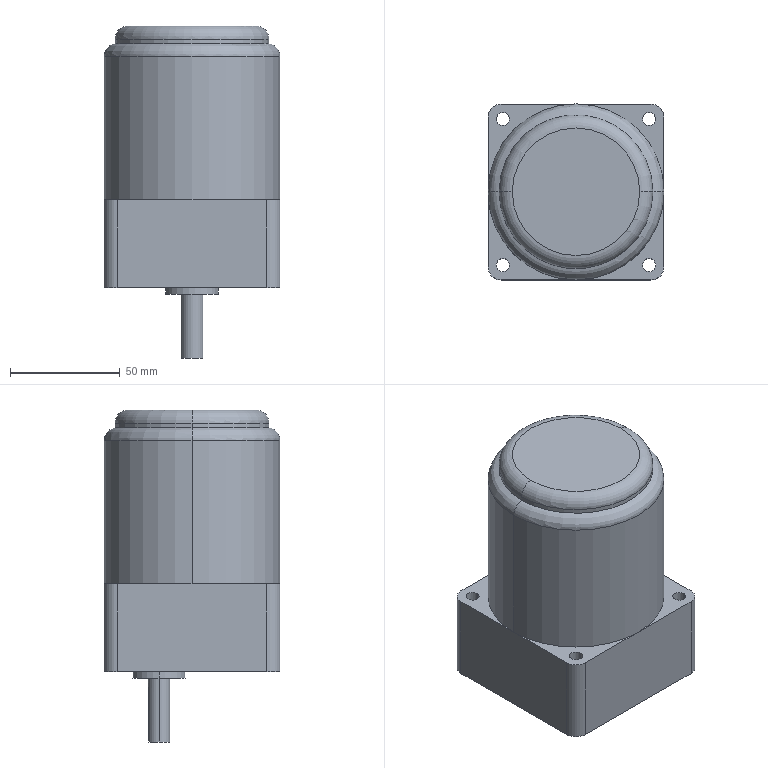Part | STEP file | 1 solid | 40 faces | box 80 x 80 x 151 mm | volume 637905 mm3 | cylinder 20 | plane 16 | torus 4 | commonest cylinder face diameters 6 x8 12 x4 10 x2 24 x2 70 x2 80 x2
STEP:
#1=CARTESIAN_POINT('',(34.,-40.,40.));
#2=VERTEX_POINT('',#1);
#3=CARTESIAN_POINT('',(0.,-40.,40.));
#4=VERTEX_POINT('',#3);
#5=CARTESIAN_POINT('',(34.,-40.,40.));
#6=DIRECTION('',(-1.,0.,0.));
#7=VECTOR('',#6,1000.);
#8=LINE('',#5,#7);
#9=EDGE_CURVE('',#2,#4,#8,.T.);
#10=ORIENTED_EDGE('',*,*,#9,.F.);
#11=CARTESIAN_POINT('',(40.,-34.,40.));
#12=VERTEX_POINT('',#11);
#13=CARTESIAN_POINT('',(34.,-34.,40.));
#14=DIRECTION('',(0.,0.,1.));
#15=DIRECTION('',(0.,-1.,0.));
#16=AXIS2_PLACEMENT_3D('',#13,#14,#15);
#17=CIRCLE('',#16,6.);
#18=EDGE_CURVE('',#2,#12,#17,.T.);
#19=ORIENTED_EDGE('',*,*,#18,.T.);
#20=CARTESIAN_POINT('',(40.,0.,40.));
#21=VERTEX_POINT('',#20);
#22=CARTESIAN_POINT('',(40.,0.,40.));
#23=DIRECTION('',(0.,-1.,0.));
#24=VECTOR('',#23,1000.);
#25=LINE('',#22,#24);
#26=EDGE_CURVE('',#21,#12,#25,.T.);
#27=ORIENTED_EDGE('',*,*,#26,.F.);
#28=CARTESIAN_POINT('',(0.,0.,40.));
#29=DIRECTION('',(0.,0.,-1.));
#30=DIRECTION('',(1.,0.,0.));
#31=AXIS2_PLACEMENT_3D('',#28,#29,#30);
#32=CIRCLE('',#31,40.);
#33=EDGE_CURVE('',#21,#4,#32,.T.);
#34=ORIENTED_EDGE('',*,*,#33,.T.);
#35=EDGE_LOOP('',(#10,#19,#27,#34));
#36=FACE_OUTER_BOUND('',#35,.T.);
#37=CARTESIAN_POINT('',(36.234,-33.234,40.));
#38=VERTEX_POINT('',#37);
#39=CARTESIAN_POINT('',(30.234,-33.234,40.));
#40=VERTEX_POINT('',#39);
#41=CARTESIAN_POINT('',(33.234,-33.234,40.));
#42=DIRECTION('',(0.,0.,-1.));
#43=DIRECTION('',(1.,0.,0.));
#44=AXIS2_PLACEMENT_3D('',#41,#42,#43);
#45=CIRCLE('',#44,3.);
#46=EDGE_CURVE('',#38,#40,#45,.T.);
#47=ORIENTED_EDGE('',*,*,#46,.T.);
#48=CARTESIAN_POINT('',(33.234,-33.234,40.));
#49=DIRECTION('',(0.,0.,-1.));
#50=DIRECTION('',(-1.,0.,0.));
#51=AXIS2_PLACEMENT_3D('',#48,#49,#50);
#52=CIRCLE('',#51,3.);
#53=EDGE_CURVE('',#40,#38,#52,.T.);
#54=ORIENTED_EDGE('',*,*,#53,.T.);
#55=EDGE_LOOP('',(#47,#54));
#56=FACE_BOUND('',#55,.T.);
#57=CARTESIAN_POINT('',(-1.06,-41.06,40.));
#58=DIRECTION('',(0.,0.,1.));
#59=DIRECTION('',(1.,0.,0.));
#60=AXIS2_PLACEMENT_3D('',#57,#58,#59);
#61=PLANE('',#60);
#62=ADVANCED_FACE('',(#36,#56),#61,.T.);
#63=CARTESIAN_POINT('',(34.,-40.,0.));
#64=VERTEX_POINT('',#63);
#65=CARTESIAN_POINT('',(-34.,-40.,0.));
#66=VERTEX_POINT('',#65);
#67=CARTESIAN_POINT('',(34.,-40.,0.));
#68=DIRECTION('',(-1.,0.,0.));
#69=VECTOR('',#68,1000.);
#70=LINE('',#67,#69);
#71=EDGE_CURVE('',#64,#66,#70,.T.);
#72=ORIENTED_EDGE('',*,*,#71,.F.);
#73=CARTESIAN_POINT('',(34.,-40.,40.));
#74=DIRECTION('',(0.,0.,-1.));
#75=VECTOR('',#74,1000.);
#76=LINE('',#73,#75);
#77=EDGE_CURVE('',#2,#64,#76,.T.);
#78=ORIENTED_EDGE('',*,*,#77,.F.);
#79=ORIENTED_EDGE('',*,*,#9,.T.);
#80=CARTESIAN_POINT('',(-34.,-40.,40.));
#81=VERTEX_POINT('',#80);
#82=CARTESIAN_POINT('',(0.,-40.,40.));
#83=DIRECTION('',(-1.,0.,0.));
#84=VECTOR('',#83,1000.);
#85=LINE('',#82,#84);
#86=EDGE_CURVE('',#4,#81,#85,.T.);
#87=ORIENTED_EDGE('',*,*,#86,.T.);
#88=CARTESIAN_POINT('',(-34.,-40.,0.));
#89=DIRECTION('',(0.,0.,1.));
#90=VECTOR('',#89,1000.);
#91=LINE('',#88,#90);
#92=EDGE_CURVE('',#66,#81,#91,.T.);
#93=ORIENTED_EDGE('',*,*,#92,.F.);
#94=EDGE_LOOP('',(#72,#78,#79,#87,#93));
#95=FACE_OUTER_BOUND('',#94,.T.);
#96=CARTESIAN_POINT('',(-35.76,-40.,-1.06));
#97=DIRECTION('',(0.,1.,0.));
#98=DIRECTION('',(0.,0.,1.));
#99=AXIS2_PLACEMENT_3D('',#96,#97,#98);
#100=PLANE('',#99);
#101=ADVANCED_FACE('',(#95),#100,.F.);
#102=ORIENTED_EDGE('',*,*,#18,.F.);
#103=ORIENTED_EDGE('',*,*,#77,.T.);
#104=CARTESIAN_POINT('',(40.,-34.,0.));
#105=VERTEX_POINT('',#104);
#106=CARTESIAN_POINT('',(34.,-34.,0.));
#107=DIRECTION('',(0.,0.,-1.));
#108=DIRECTION('',(1.,0.,0.));
#109=AXIS2_PLACEMENT_3D('',#106,#107,#108);
#110=CIRCLE('',#109,6.);
#111=EDGE_CURVE('',#105,#64,#110,.T.);
#112=ORIENTED_EDGE('',*,*,#111,.F.);
#113=CARTESIAN_POINT('',(40.,-34.,0.));
#114=DIRECTION('',(0.,0.,1.));
#115=VECTOR('',#114,1000.);
#116=LINE('',#113,#115);
#117=EDGE_CURVE('',#105,#12,#116,.T.);
#118=ORIENTED_EDGE('',*,*,#117,.T.);
#119=EDGE_LOOP('',(#102,#103,#112,#118));
#120=FACE_OUTER_BOUND('',#119,.T.);
#121=CARTESIAN_POINT('',(34.,-34.,40.5));
#122=DIRECTION('',(0.,0.,-1.));
#123=DIRECTION('',(0.9987,0.05123,0.));
#124=AXIS2_PLACEMENT_3D('',#121,#122,#123);
#125=CYLINDRICAL_SURFACE('',#124,6.);
#126=ADVANCED_FACE('',(#120),#125,.T.);
#127=ORIENTED_EDGE('',*,*,#26,.T.);
#128=ORIENTED_EDGE('',*,*,#117,.F.);
#129=CARTESIAN_POINT('',(40.,34.,0.));
#130=VERTEX_POINT('',#129);
#131=CARTESIAN_POINT('',(40.,34.,0.));
#132=DIRECTION('',(0.,-1.,0.));
#133=VECTOR('',#132,1000.);
#134=LINE('',#131,#133);
#135=EDGE_CURVE('',#130,#105,#134,.T.);
#136=ORIENTED_EDGE('',*,*,#135,.F.);
#137=CARTESIAN_POINT('',(40.,34.,40.));
#138=VERTEX_POINT('',#137);
#139=CARTESIAN_POINT('',(40.,34.,40.));
#140=DIRECTION('',(0.,0.,-1.));
#141=VECTOR('',#140,1000.);
#142=LINE('',#139,#141);
#143=EDGE_CURVE('',#138,#130,#142,.T.);
#144=ORIENTED_EDGE('',*,*,#143,.F.);
#145=CARTESIAN_POINT('',(40.,34.,40.));
#146=DIRECTION('',(0.,-1.,0.));
#147=VECTOR('',#146,1000.);
#148=LINE('',#145,#147);
#149=EDGE_CURVE('',#138,#21,#148,.T.);
#150=ORIENTED_EDGE('',*,*,#149,.T.);
#151=EDGE_LOOP('',(#127,#128,#136,#144,#150));
#152=FACE_OUTER_BOUND('',#151,.T.);
#153=CARTESIAN_POINT('',(40.,35.76,-1.06));
#154=DIRECTION('',(-1.,0.,0.));
#155=DIRECTION('',(0.,-1.,0.));
#156=AXIS2_PLACEMENT_3D('',#153,#154,#155);
#157=PLANE('',#156);
#158=ADVANCED_FACE('',(#152),#157,.F.);
#159=CARTESIAN_POINT('',(-40.,0.,105.084));
#160=VERTEX_POINT('',#159);
#161=CARTESIAN_POINT('',(-40.,0.,40.));
#162=VERTEX_POINT('',#161);
#163=CARTESIAN_POINT('',(-40.,0.,105.084));
#164=DIRECTION('',(0.,0.,-1.));
#165=VECTOR('',#164,1000.);
#166=LINE('',#163,#165);
#167=EDGE_CURVE('',#160,#162,#166,.T.);
#168=ORIENTED_EDGE('',*,*,#167,.T.);
#169=CARTESIAN_POINT('',(0.,0.,40.));
#170=DIRECTION('',(0.,0.,-1.));
#171=DIRECTION('',(0.,-1.,0.));
#172=AXIS2_PLACEMENT_3D('',#169,#170,#171);
#173=CIRCLE('',#172,40.);
#174=EDGE_CURVE('',#4,#162,#173,.T.);
#175=ORIENTED_EDGE('',*,*,#174,.F.);
#176=ORIENTED_EDGE('',*,*,#33,.F.);
#177=CARTESIAN_POINT('',(40.,0.,105.084));
#178=VERTEX_POINT('',#177);
#179=CARTESIAN_POINT('',(40.,0.,105.084));
#180=DIRECTION('',(0.,0.,-1.));
#181=VECTOR('',#180,1000.);
#182=LINE('',#179,#181);
#183=EDGE_CURVE('',#178,#21,#182,.T.);
#184=ORIENTED_EDGE('',*,*,#183,.F.);
#185=CARTESIAN_POINT('',(0.,0.,105.084));
#186=DIRECTION('',(0.,0.,1.));
#187=DIRECTION('',(-1.,0.,0.));
#188=AXIS2_PLACEMENT_3D('',#185,#186,#187);
#189=CIRCLE('',#188,40.);
#190=EDGE_CURVE('',#160,#178,#189,.T.);
#191=ORIENTED_EDGE('',*,*,#190,.F.);
#192=EDGE_LOOP('',(#168,#175,#176,#184,#191));
#193=FACE_OUTER_BOUND('',#192,.T.);
#194=CARTESIAN_POINT('',(0.,0.,105.584));
#195=DIRECTION('',(0.,0.,-1.));
#196=DIRECTION('',(0.9946,0.1036,0.));
#197=AXIS2_PLACEMENT_3D('',#194,#195,#196);
#198=CYLINDRICAL_SURFACE('',#197,40.);
#199=ADVANCED_FACE('',(#193),#198,.T.);
#200=ORIENTED_EDGE('',*,*,#46,.F.);
#201=CARTESIAN_POINT('',(36.234,-33.234,0.));
#202=VERTEX_POINT('',#201);
#203=CARTESIAN_POINT('',(36.234,-33.234,40.));
#204=DIRECTION('',(0.,0.,-1.));
#205=VECTOR('',#204,1000.);
#206=LINE('',#203,#205);
#207=EDGE_CURVE('',#38,#202,#206,.T.);
#208=ORIENTED_EDGE('',*,*,#207,.T.);
#209=CARTESIAN_POINT('',(30.234,-33.234,0.));
#210=VERTEX_POINT('',#209);
#211=CARTESIAN_POINT('',(33.234,-33.234,0.));
#212=DIRECTION('',(0.,0.,1.));
#213=DIRECTION('',(-1.,0.,0.));
#214=AXIS2_PLACEMENT_3D('',#211,#212,#213);
#215=CIRCLE('',#214,3.);
#216=EDGE_CURVE('',#210,#202,#215,.T.);
#217=ORIENTED_EDGE('',*,*,#216,.F.);
#218=CARTESIAN_POINT('',(30.234,-33.234,40.));
#219=DIRECTION('',(0.,0.,-1.));
#220=VECTOR('',#219,1000.);
#221=LINE('',#218,#220);
#222=EDGE_CURVE('',#40,#210,#221,.T.);
#223=ORIENTED_EDGE('',*,*,#222,.F.);
#224=EDGE_LOOP('',(#200,#208,#217,#223));
#225=FACE_OUTER_BOUND('',#224,.T.);
#226=CARTESIAN_POINT('',(33.234,-33.234,40.5));
#227=DIRECTION('',(0.,0.,-1.));
#228=DIRECTION('',(0.9946,0.1036,0.));
#229=AXIS2_PLACEMENT_3D('',#226,#227,#228);
#230=CYLINDRICAL_SURFACE('',#229,3.);
#231=ADVANCED_FACE('',(#225),#230,.F.);
#232=CARTESIAN_POINT('',(33.234,-33.234,0.));
#233=DIRECTION('',(0.,0.,1.));
#234=DIRECTION('',(1.,0.,0.));
#235=AXIS2_PLACEMENT_3D('',#232,#233,#234);
#236=CIRCLE('',#235,3.);
#237=EDGE_CURVE('',#202,#210,#236,.T.);
#238=ORIENTED_EDGE('',*,*,#237,.F.);
#239=ORIENTED_EDGE('',*,*,#207,.F.);
#240=ORIENTED_EDGE('',*,*,#53,.F.);
#241=ORIENTED_EDGE('',*,*,#222,.T.);
#242=EDGE_LOOP('',(#238,#239,#240,#241));
#243=FACE_OUTER_BOUND('',#242,.T.);
#244=CARTESIAN_POINT('',(33.234,-33.234,40.5));
#245=DIRECTION('',(0.,0.,-1.));
#246=DIRECTION('',(-0.9993,-0.03732,0.));
#247=AXIS2_PLACEMENT_3D('',#244,#245,#246);
#248=CYLINDRICAL_SURFACE('',#247,3.);
#249=ADVANCED_FACE('',(#243),#248,.F.);
#250=CARTESIAN_POINT('',(-40.,-34.,40.));
#251=VERTEX_POINT('',#250);
#252=CARTESIAN_POINT('',(-34.,-34.,40.));
#253=DIRECTION('',(0.,0.,1.));
#254=DIRECTION('',(-1.,0.,0.));
#255=AXIS2_PLACEMENT_3D('',#252,#253,#254);
#256=CIRCLE('',#255,6.);
#257=EDGE_CURVE('',#251,#81,#256,.T.);
#258=ORIENTED_EDGE('',*,*,#257,.F.);
#259=CARTESIAN_POINT('',(-40.,-34.,0.));
#260=VERTEX_POINT('',#259);
#261=CARTESIAN_POINT('',(-40.,-34.,40.));
#262=DIRECTION('',(0.,0.,-1.));
#263=VECTOR('',#262,1000.);
#264=LINE('',#261,#263);
#265=EDGE_CURVE('',#251,#260,#264,.T.);
#266=ORIENTED_EDGE('',*,*,#265,.T.);
#267=CARTESIAN_POINT('',(-34.,-34.,0.));
#268=DIRECTION('',(0.,0.,-1.));
#269=DIRECTION('',(0.,-1.,0.));
#270=AXIS2_PLACEMENT_3D('',#267,#268,#269);
#271=CIRCLE('',#270,6.);
#272=EDGE_CURVE('',#66,#260,#271,.T.);
#273=ORIENTED_EDGE('',*,*,#272,.F.);
#274=ORIENTED_EDGE('',*,*,#92,.T.);
#275=EDGE_LOOP('',(#258,#266,#273,#274));
#276=FACE_OUTER_BOUND('',#275,.T.);
#277=CARTESIAN_POINT('',(-34.,-34.,40.5));
#278=DIRECTION('',(0.,0.,-1.));
#279=DIRECTION('',(0.05123,-0.9987,0.));
#280=AXIS2_PLACEMENT_3D('',#277,#278,#279);
#281=CYLINDRICAL_SURFACE('',#280,6.);
#282=ADVANCED_FACE('',(#276),#281,.T.);
#283=CARTESIAN_POINT('',(-40.,-34.,40.));
#284=DIRECTION('',(0.,1.,0.));
#285=VECTOR('',#284,1000.);
#286=LINE('',#283,#285);
#287=EDGE_CURVE('',#251,#162,#286,.T.);
#288=ORIENTED_EDGE('',*,*,#287,.F.);
#289=ORIENTED_EDGE('',*,*,#257,.T.);
#290=ORIENTED_EDGE('',*,*,#86,.F.);
#291=ORIENTED_EDGE('',*,*,#174,.T.);
#292=EDGE_LOOP('',(#288,#289,#290,#291));
#293=FACE_OUTER_BOUND('',#292,.T.);
#294=CARTESIAN_POINT('',(-36.234,-33.234,40.));
#295=VERTEX_POINT('',#294);
#296=CARTESIAN_POINT('',(-30.234,-33.234,40.));
#297=VERTEX_POINT('',#296);
#298=CARTESIAN_POINT('',(-33.234,-33.234,40.));
#299=DIRECTION('',(0.,0.,-1.));
#300=DIRECTION('',(-1.,0.,0.));
#301=AXIS2_PLACEMENT_3D('',#298,#299,#300);
#302=CIRCLE('',#301,3.);
#303=EDGE_CURVE('',#295,#297,#302,.T.);
#304=ORIENTED_EDGE('',*,*,#303,.T.);
#305=CARTESIAN_POINT('',(-33.234,-33.234,40.));
#306=DIRECTION('',(0.,0.,-1.));
#307=DIRECTION('',(1.,0.,0.));
#308=AXIS2_PLACEMENT_3D('',#305,#306,#307);
#309=CIRCLE('',#308,3.);
#310=EDGE_CURVE('',#297,#295,#309,.T.);
#311=ORIENTED_EDGE('',*,*,#310,.T.);
#312=EDGE_LOOP('',(#304,#311));
#313=FACE_BOUND('',#312,.T.);
#314=CARTESIAN_POINT('',(-41.06,-41.06,40.));
#315=DIRECTION('',(0.,0.,1.));
#316=DIRECTION('',(1.,0.,0.));
#317=AXIS2_PLACEMENT_3D('',#314,#315,#316);
#318=PLANE('',#317);
#319=ADVANCED_FACE('',(#293,#313),#318,.T.);
#320=ORIENTED_EDGE('',*,*,#135,.T.);
#321=ORIENTED_EDGE('',*,*,#111,.T.);
#322=ORIENTED_EDGE('',*,*,#71,.T.);
#323=ORIENTED_EDGE('',*,*,#272,.T.);
#324=CARTESIAN_POINT('',(-40.,34.,0.));
#325=VERTEX_POINT('',#324);
#326=CARTESIAN_POINT('',(-40.,-34.,0.));
#327=DIRECTION('',(0.,1.,0.));
#328=VECTOR('',#327,1000.);
#329=LINE('',#326,#328);
#330=EDGE_CURVE('',#260,#325,#329,.T.);
#331=ORIENTED_EDGE('',*,*,#330,.T.);
#332=CARTESIAN_POINT('',(-34.,40.,0.));
#333=VERTEX_POINT('',#332);
#334=CARTESIAN_POINT('',(-34.,34.,0.));
#335=DIRECTION('',(0.,0.,-1.));
#336=DIRECTION('',(-1.,0.,0.));
#337=AXIS2_PLACEMENT_3D('',#334,#335,#336);
#338=CIRCLE('',#337,6.);
#339=EDGE_CURVE('',#325,#333,#338,.T.);
#340=ORIENTED_EDGE('',*,*,#339,.T.);
#341=CARTESIAN_POINT('',(34.,40.,0.));
#342=VERTEX_POINT('',#341);
#343=CARTESIAN_POINT('',(-34.,40.,0.));
#344=DIRECTION('',(1.,0.,0.));
#345=VECTOR('',#344,1000.);
#346=LINE('',#343,#345);
#347=EDGE_CURVE('',#333,#342,#346,.T.);
#348=ORIENTED_EDGE('',*,*,#347,.T.);
#349=CARTESIAN_POINT('',(34.,34.,0.));
#350=DIRECTION('',(0.,0.,-1.));
#351=DIRECTION('',(0.,1.,0.));
#352=AXIS2_PLACEMENT_3D('',#349,#350,#351);
#353=CIRCLE('',#352,6.);
#354=EDGE_CURVE('',#342,#130,#353,.T.);
#355=ORIENTED_EDGE('',*,*,#354,.T.);
#356=EDGE_LOOP('',(#320,#321,#322,#323,#331,#340,#348,#355));
#357=FACE_OUTER_BOUND('',#356,.T.);
#358=CARTESIAN_POINT('',(-30.234,33.234,0.));
#359=VERTEX_POINT('',#358);
#360=CARTESIAN_POINT('',(-36.234,33.234,0.));
#361=VERTEX_POINT('',#360);
#362=CARTESIAN_POINT('',(-33.234,33.234,0.));
#363=DIRECTION('',(0.,0.,1.));
#364=DIRECTION('',(1.,0.,0.));
#365=AXIS2_PLACEMENT_3D('',#362,#363,#364);
#366=CIRCLE('',#365,3.);
#367=EDGE_CURVE('',#359,#361,#366,.T.);
#368=ORIENTED_EDGE('',*,*,#367,.T.);
#369=CARTESIAN_POINT('',(-33.234,33.234,0.));
#370=DIRECTION('',(0.,0.,1.));
#371=DIRECTION('',(-1.,0.,0.));
#372=AXIS2_PLACEMENT_3D('',#369,#370,#371);
#373=CIRCLE('',#372,3.);
#374=EDGE_CURVE('',#361,#359,#373,.T.);
#375=ORIENTED_EDGE('',*,*,#374,.T.);
#376=EDGE_LOOP('',(#368,#375));
#377=FACE_BOUND('',#376,.T.);
#378=CARTESIAN_POINT('',(-30.234,-33.234,0.));
#379=VERTEX_POINT('',#378);
#380=CARTESIAN_POINT('',(-36.234,-33.234,0.));
#381=VERTEX_POINT('',#380);
#382=CARTESIAN_POINT('',(-33.234,-33.234,0.));
#383=DIRECTION('',(0.,0.,1.));
#384=DIRECTION('',(1.,0.,0.));
#385=AXIS2_PLACEMENT_3D('',#382,#383,#384);
#386=CIRCLE('',#385,3.);
#387=EDGE_CURVE('',#379,#381,#386,.T.);
#388=ORIENTED_EDGE('',*,*,#387,.T.);
#389=CARTESIAN_POINT('',(-33.234,-33.234,0.));
#390=DIRECTION('',(0.,0.,1.));
#391=DIRECTION('',(-1.,0.,0.));
#392=AXIS2_PLACEMENT_3D('',#389,#390,#391);
#393=CIRCLE('',#392,3.);
#394=EDGE_CURVE('',#381,#379,#393,.T.);
#395=ORIENTED_EDGE('',*,*,#394,.T.);
#396=EDGE_LOOP('',(#388,#395));
#397=FACE_BOUND('',#396,.T.);
#398=ORIENTED_EDGE('',*,*,#237,.T.);
#399=ORIENTED_EDGE('',*,*,#216,.T.);
#400=EDGE_LOOP('',(#398,#399));
#401=FACE_BOUND('',#400,.T.);
#402=CARTESIAN_POINT('',(30.234,33.234,0.));
#403=VERTEX_POINT('',#402);
#404=CARTESIAN_POINT('',(36.234,33.234,0.));
#405=VERTEX_POINT('',#404);
#406=CARTESIAN_POINT('',(33.234,33.234,0.));
#407=DIRECTION('',(0.,0.,1.));
#408=DIRECTION('',(-1.,0.,0.));
#409=AXIS2_PLACEMENT_3D('',#406,#407,#408);
#410=CIRCLE('',#409,3.);
#411=EDGE_CURVE('',#403,#405,#410,.T.);
#412=ORIENTED_EDGE('',*,*,#411,.T.);
#413=CARTESIAN_POINT('',(33.234,33.234,0.));
#414=DIRECTION('',(0.,0.,1.));
#415=DIRECTION('',(1.,0.,0.));
#416=AXIS2_PLACEMENT_3D('',#413,#414,#415);
#417=CIRCLE('',#416,3.);
#418=EDGE_CURVE('',#405,#403,#417,.T.);
#419=ORIENTED_EDGE('',*,*,#418,.T.);
#420=EDGE_LOOP('',(#412,#419));
#421=FACE_BOUND('',#420,.T.);
#422=CARTESIAN_POINT('',(-12.,15.,0.));
#423=VERTEX_POINT('',#422);
#424=CARTESIAN_POINT('',(12.,15.,0.));
#425=VERTEX_POINT('',#424);
#426=CARTESIAN_POINT('',(0.,15.,0.));
#427=DIRECTION('',(0.,0.,1.));
#428=DIRECTION('',(-1.,0.,0.));
#429=AXIS2_PLACEMENT_3D('',#426,#427,#428);
#430=CIRCLE('',#429,12.);
#431=EDGE_CURVE('',#423,#425,#430,.T.);
#432=ORIENTED_EDGE('',*,*,#431,.T.);
#433=CARTESIAN_POINT('',(0.,15.,0.));
#434=DIRECTION('',(0.,0.,1.));
#435=DIRECTION('',(1.,0.,0.));
#436=AXIS2_PLACEMENT_3D('',#433,#434,#435);
#437=CIRCLE('',#436,12.);
#438=EDGE_CURVE('',#425,#423,#437,.T.);
#439=ORIENTED_EDGE('',*,*,#438,.T.);
#440=EDGE_LOOP('',(#432,#439));
#441=FACE_BOUND('',#440,.T.);
#442=CARTESIAN_POINT('',(-42.06,-42.06,0.));
#443=DIRECTION('',(0.,0.,1.));
#444=DIRECTION('',(1.,0.,0.));
#445=AXIS2_PLACEMENT_3D('',#442,#443,#444);
#446=PLANE('',#445);
#447=ADVANCED_FACE('',(#357,#377,#397,#401,#421,#441),#446,.F.);
#448=ORIENTED_EDGE('',*,*,#149,.F.);
#449=CARTESIAN_POINT('',(34.,40.,40.));
#450=VERTEX_POINT('',#449);
#451=CARTESIAN_POINT('',(34.,34.,40.));
#452=DIRECTION('',(0.,0.,1.));
#453=DIRECTION('',(1.,0.,0.));
#454=AXIS2_PLACEMENT_3D('',#451,#452,#453);
#455=CIRCLE('',#454,6.);
#456=EDGE_CURVE('',#138,#450,#455,.T.);
#457=ORIENTED_EDGE('',*,*,#456,.T.);
#458=CARTESIAN_POINT('',(0.,40.,40.));
#459=VERTEX_POINT('',#458);
#460=CARTESIAN_POINT('',(0.,40.,40.));
#461=DIRECTION('',(1.,0.,0.));
#462=VECTOR('',#461,1000.);
#463=LINE('',#460,#462);
#464=EDGE_CURVE('',#459,#450,#463,.T.);
#465=ORIENTED_EDGE('',*,*,#464,.F.);
#466=CARTESIAN_POINT('',(0.,0.,40.));
#467=DIRECTION('',(0.,0.,-1.));
#468=DIRECTION('',(0.,1.,0.));
#469=AXIS2_PLACEMENT_3D('',#466,#467,#468);
#470=CIRCLE('',#469,40.);
#471=EDGE_CURVE('',#459,#21,#470,.T.);
#472=ORIENTED_EDGE('',*,*,#471,.T.);
#473=EDGE_LOOP('',(#448,#457,#465,#472));
#474=FACE_OUTER_BOUND('',#473,.T.);
#475=CARTESIAN_POINT('',(30.234,33.234,40.));
#476=VERTEX_POINT('',#475);
#477=CARTESIAN_POINT('',(36.234,33.234,40.));
#478=VERTEX_POINT('',#477);
#479=CARTESIAN_POINT('',(33.234,33.234,40.));
#480=DIRECTION('',(0.,0.,-1.));
#481=DIRECTION('',(-1.,0.,0.));
#482=AXIS2_PLACEMENT_3D('',#479,#480,#481);
#483=CIRCLE('',#482,3.);
#484=EDGE_CURVE('',#476,#478,#483,.T.);
#485=ORIENTED_EDGE('',*,*,#484,.T.);
#486=CARTESIAN_POINT('',(33.234,33.234,40.));
#487=DIRECTION('',(0.,0.,-1.));
#488=DIRECTION('',(1.,0.,0.));
#489=AXIS2_PLACEMENT_3D('',#486,#487,#488);
#490=CIRCLE('',#489,3.);
#491=EDGE_CURVE('',#478,#476,#490,.T.);
#492=ORIENTED_EDGE('',*,*,#491,.T.);
#493=EDGE_LOOP('',(#485,#492));
#494=FACE_BOUND('',#493,.T.);
#495=CARTESIAN_POINT('',(-1.06,-1.06,40.));
#496=DIRECTION('',(0.,0.,1.));
#497=DIRECTION('',(1.,0.,0.));
#498=AXIS2_PLACEMENT_3D('',#495,#496,#497);
#499=PLANE('',#498);
#500=ADVANCED_FACE('',(#474,#494),#499,.T.);
#501=ORIENTED_EDGE('',*,*,#456,.F.);
#502=ORIENTED_EDGE('',*,*,#143,.T.);
#503=ORIENTED_EDGE('',*,*,#354,.F.);
#504=CARTESIAN_POINT('',(34.,40.,0.));
#505=DIRECTION('',(0.,0.,1.));
#506=VECTOR('',#505,1000.);
#507=LINE('',#504,#506);
#508=EDGE_CURVE('',#342,#450,#507,.T.);
#509=ORIENTED_EDGE('',*,*,#508,.T.);
#510=EDGE_LOOP('',(#501,#502,#503,#509));
#511=FACE_OUTER_BOUND('',#510,.T.);
#512=CARTESIAN_POINT('',(34.,34.,40.5));
#513=DIRECTION('',(0.,0.,-1.));
#514=DIRECTION('',(-0.05123,0.9987,0.));
#515=AXIS2_PLACEMENT_3D('',#512,#513,#514);
#516=CYLINDRICAL_SURFACE('',#515,6.);
#517=ADVANCED_FACE('',(#511),#516,.T.);
#518=ORIENTED_EDGE('',*,*,#167,.F.);
#519=CARTESIAN_POINT('',(0.,0.,105.084));
#520=DIRECTION('',(0.,0.,1.));
#521=DIRECTION('',(1.,0.,0.));
#522=AXIS2_PLACEMENT_3D('',#519,#520,#521);
#523=CIRCLE('',#522,40.);
#524=EDGE_CURVE('',#178,#160,#523,.T.);
#525=ORIENTED_EDGE('',*,*,#524,.F.);
#526=ORIENTED_EDGE('',*,*,#183,.T.);
#527=ORIENTED_EDGE('',*,*,#471,.F.);
#528=CARTESIAN_POINT('',(0.,0.,40.));
#529=DIRECTION('',(0.,0.,-1.));
#530=DIRECTION('',(-1.,0.,0.));
#531=AXIS2_PLACEMENT_3D('',#528,#529,#530);
#532=CIRCLE('',#531,40.);
#533=EDGE_CURVE('',#162,#459,#532,.T.);
#534=ORIENTED_EDGE('',*,*,#533,.F.);
#535=EDGE_LOOP('',(#518,#525,#526,#527,#534));
#536=FACE_OUTER_BOUND('',#535,.T.);
#537=CARTESIAN_POINT('',(0.,0.,105.584));
#538=DIRECTION('',(0.,0.,-1.));
#539=DIRECTION('',(-1.,-0.0028,0.));
#540=AXIS2_PLACEMENT_3D('',#537,#538,#539);
#541=CYLINDRICAL_SURFACE('',#540,40.);
#542=ADVANCED_FACE('',(#536),#541,.T.);
#543=CARTESIAN_POINT('',(35.,0.,111.));
#544=VERTEX_POINT('',#543);
#545=CARTESIAN_POINT('',(34.,0.,105.084));
#546=DIRECTION('',(0.,1.,0.));
#547=DIRECTION('',(0.1667,0.,0.986));
#548=AXIS2_PLACEMENT_3D('',#545,#546,#547);
#549=CIRCLE('',#548,6.);
#550=EDGE_CURVE('',#544,#178,#549,.T.);
#551=ORIENTED_EDGE('',*,*,#550,.F.);
#552=CARTESIAN_POINT('',(-35.,0.,111.));
#553=VERTEX_POINT('',#552);
#554=CARTESIAN_POINT('',(0.,0.,111.));
#555=DIRECTION('',(0.,0.,-1.));
#556=DIRECTION('',(1.,0.,0.));
#557=AXIS2_PLACEMENT_3D('',#554,#555,#556);
#558=CIRCLE('',#557,35.);
#559=EDGE_CURVE('',#544,#553,#558,.T.);
#560=ORIENTED_EDGE('',*,*,#559,.T.);
#561=CARTESIAN_POINT('',(-34.,0.,105.084));
#562=DIRECTION('',(0.,-1.,0.));
#563=DIRECTION('',(-0.1667,0.,0.986));
#564=AXIS2_PLACEMENT_3D('',#561,#562,#563);
#565=CIRCLE('',#564,6.);
#566=EDGE_CURVE('',#553,#160,#565,.T.);
#567=ORIENTED_EDGE('',*,*,#566,.T.);
#568=ORIENTED_EDGE('',*,*,#190,.T.);
#569=EDGE_LOOP('',(#551,#560,#567,#568));
#570=FACE_OUTER_BOUND('',#569,.T.);
#571=CARTESIAN_POINT('',(0.,0.,105.084));
#572=DIRECTION('',(0.,0.,-1.));
#573=DIRECTION('',(1.,0.004335,0.));
#574=AXIS2_PLACEMENT_3D('',#571,#572,#573);
#575=TOROIDAL_SURFACE('',#574,34.,6.);
#576=ADVANCED_FACE('',(#570),#575,.T.);
#577=ORIENTED_EDGE('',*,*,#330,.F.);
#578=ORIENTED_EDGE('',*,*,#265,.F.);
#579=ORIENTED_EDGE('',*,*,#287,.T.);
#580=CARTESIAN_POINT('',(-40.,34.,40.));
#581=VERTEX_POINT('',#580);
#582=CARTESIAN_POINT('',(-40.,0.,40.));
#583=DIRECTION('',(0.,1.,0.));
#584=VECTOR('',#583,1000.);
#585=LINE('',#582,#584);
#586=EDGE_CURVE('',#162,#581,#585,.T.);
#587=ORIENTED_EDGE('',*,*,#586,.T.);
#588=CARTESIAN_POINT('',(-40.,34.,0.));
#589=DIRECTION('',(0.,0.,1.));
#590=VECTOR('',#589,1000.);
#591=LINE('',#588,#590);
#592=EDGE_CURVE('',#325,#581,#591,.T.);
#593=ORIENTED_EDGE('',*,*,#592,.F.);
#594=EDGE_LOOP('',(#577,#578,#579,#587,#593));
#595=FACE_OUTER_BOUND('',#594,.T.);
#596=CARTESIAN_POINT('',(-40.,-35.76,-1.06));
#597=DIRECTION('',(1.,0.,0.));
#598=DIRECTION('',(0.,1.,0.));
#599=AXIS2_PLACEMENT_3D('',#596,#597,#598);
#600=PLANE('',#599);
#601=ADVANCED_FACE('',(#595),#600,.F.);
#602=ORIENTED_EDGE('',*,*,#387,.F.);
#603=CARTESIAN_POINT('',(-30.234,-33.234,40.));
#604=DIRECTION('',(0.,0.,-1.));
#605=VECTOR('',#604,1000.);
#606=LINE('',#603,#605);
#607=EDGE_CURVE('',#297,#379,#606,.T.);
#608=ORIENTED_EDGE('',*,*,#607,.F.);
#609=ORIENTED_EDGE('',*,*,#303,.F.);
#610=CARTESIAN_POINT('',(-36.234,-33.234,40.));
#611=DIRECTION('',(0.,0.,-1.));
#612=VECTOR('',#611,1000.);
#613=LINE('',#610,#612);
#614=EDGE_CURVE('',#295,#381,#613,.T.);
#615=ORIENTED_EDGE('',*,*,#614,.T.);
#616=EDGE_LOOP('',(#602,#608,#609,#615));
#617=FACE_OUTER_BOUND('',#616,.T.);
#618=CARTESIAN_POINT('',(-33.234,-33.234,40.5));
#619=DIRECTION('',(0.,0.,-1.));
#620=DIRECTION('',(-0.9993,-0.03732,0.));
#621=AXIS2_PLACEMENT_3D('',#618,#619,#620);
#622=CYLINDRICAL_SURFACE('',#621,3.);
#623=ADVANCED_FACE('',(#617),#622,.F.);
#624=ORIENTED_EDGE('',*,*,#310,.F.);
#625=ORIENTED_EDGE('',*,*,#607,.T.);
#626=ORIENTED_EDGE('',*,*,#394,.F.);
#627=ORIENTED_EDGE('',*,*,#614,.F.);
#628=EDGE_LOOP('',(#624,#625,#626,#627));
#629=FACE_OUTER_BOUND('',#628,.T.);
#630=CARTESIAN_POINT('',(-33.234,-33.234,40.5));
#631=DIRECTION('',(0.,0.,-1.));
#632=DIRECTION('',(0.9946,0.1036,0.));
#633=AXIS2_PLACEMENT_3D('',#630,#631,#632);
#634=CYLINDRICAL_SURFACE('',#633,3.);
#635=ADVANCED_FACE('',(#629),#634,.F.);
#636=ORIENTED_EDGE('',*,*,#347,.F.);
#637=CARTESIAN_POINT('',(-34.,40.,40.));
#638=VERTEX_POINT('',#637);
#639=CARTESIAN_POINT('',(-34.,40.,40.));
#640=DIRECTION('',(0.,0.,-1.));
#641=VECTOR('',#640,1000.);
#642=LINE('',#639,#641);
#643=EDGE_CURVE('',#638,#333,#642,.T.);
#644=ORIENTED_EDGE('',*,*,#643,.F.);
#645=CARTESIAN_POINT('',(-34.,40.,40.));
#646=DIRECTION('',(1.,0.,0.));
#647=VECTOR('',#646,1000.);
#648=LINE('',#645,#647);
#649=EDGE_CURVE('',#638,#459,#648,.T.);
#650=ORIENTED_EDGE('',*,*,#649,.T.);
#651=ORIENTED_EDGE('',*,*,#464,.T.);
#652=ORIENTED_EDGE('',*,*,#508,.F.);
#653=EDGE_LOOP('',(#636,#644,#650,#651,#652));
#654=FACE_OUTER_BOUND('',#653,.T.);
#655=CARTESIAN_POINT('',(-35.76,40.,41.06));
#656=DIRECTION('',(0.,-1.,0.));
#657=DIRECTION('',(0.,0.,-1.));
#658=AXIS2_PLACEMENT_3D('',#655,#656,#657);
#659=PLANE('',#658);
#660=ADVANCED_FACE('',(#654),#659,.F.);
#661=CARTESIAN_POINT('',(-34.,34.,40.));
#662=DIRECTION('',(0.,0.,1.));
#663=DIRECTION('',(0.,1.,0.));
#664=AXIS2_PLACEMENT_3D('',#661,#662,#663);
#665=CIRCLE('',#664,6.);
#666=EDGE_CURVE('',#638,#581,#665,.T.);
#667=ORIENTED_EDGE('',*,*,#666,.F.);
#668=ORIENTED_EDGE('',*,*,#643,.T.);
#669=ORIENTED_EDGE('',*,*,#339,.F.);
#670=ORIENTED_EDGE('',*,*,#592,.T.);
#671=EDGE_LOOP('',(#667,#668,#669,#670));
#672=FACE_OUTER_BOUND('',#671,.T.);
#673=CARTESIAN_POINT('',(-34.,34.,40.5));
#674=DIRECTION('',(0.,0.,-1.));
#675=DIRECTION('',(-0.9987,-0.05123,0.));
#676=AXIS2_PLACEMENT_3D('',#673,#674,#675);
#677=CYLINDRICAL_SURFACE('',#676,6.);
#678=ADVANCED_FACE('',(#672),#677,.T.);
#679=CARTESIAN_POINT('',(-30.234,33.234,40.));
#680=VERTEX_POINT('',#679);
#681=CARTESIAN_POINT('',(-36.234,33.234,40.));
#682=VERTEX_POINT('',#681);
#683=CARTESIAN_POINT('',(-33.234,33.234,40.));
#684=DIRECTION('',(0.,0.,-1.));
#685=DIRECTION('',(1.,0.,0.));
#686=AXIS2_PLACEMENT_3D('',#683,#684,#685);
#687=CIRCLE('',#686,3.);
#688=EDGE_CURVE('',#680,#682,#687,.T.);
#689=ORIENTED_EDGE('',*,*,#688,.F.);
#690=CARTESIAN_POINT('',(-30.234,33.234,40.));
#691=DIRECTION('',(0.,0.,-1.));
#692=VECTOR('',#691,1000.);
#693=LINE('',#690,#692);
#694=EDGE_CURVE('',#680,#359,#693,.T.);
#695=ORIENTED_EDGE('',*,*,#694,.T.);
#696=ORIENTED_EDGE('',*,*,#374,.F.);
#697=CARTESIAN_POINT('',(-36.234,33.234,40.));
#698=DIRECTION('',(0.,0.,-1.));
#699=VECTOR('',#698,1000.);
#700=LINE('',#697,#699);
#701=EDGE_CURVE('',#682,#361,#700,.T.);
#702=ORIENTED_EDGE('',*,*,#701,.F.);
#703=EDGE_LOOP('',(#689,#695,#696,#702));
#704=FACE_OUTER_BOUND('',#703,.T.);
#705=CARTESIAN_POINT('',(-33.234,33.234,40.5));
#706=DIRECTION('',(0.,0.,-1.));
#707=DIRECTION('',(0.9946,0.1036,0.));
#708=AXIS2_PLACEMENT_3D('',#705,#706,#707);
#709=CYLINDRICAL_SURFACE('',#708,3.);
#710=ADVANCED_FACE('',(#704),#709,.F.);
#711=ORIENTED_EDGE('',*,*,#367,.F.);
#712=ORIENTED_EDGE('',*,*,#694,.F.);
#713=CARTESIAN_POINT('',(-33.234,33.234,40.));
#714=DIRECTION('',(0.,0.,-1.));
#715=DIRECTION('',(-1.,0.,0.));
#716=AXIS2_PLACEMENT_3D('',#713,#714,#715);
#717=CIRCLE('',#716,3.);
#718=EDGE_CURVE('',#682,#680,#717,.T.);
#719=ORIENTED_EDGE('',*,*,#718,.F.);
#720=ORIENTED_EDGE('',*,*,#701,.T.);
#721=EDGE_LOOP('',(#711,#712,#719,#720));
#722=FACE_OUTER_BOUND('',#721,.T.);
#723=CARTESIAN_POINT('',(-33.234,33.234,40.5));
#724=DIRECTION('',(0.,0.,-1.));
#725=DIRECTION('',(-0.9993,-0.03732,0.));
#726=AXIS2_PLACEMENT_3D('',#723,#724,#725);
#727=CYLINDRICAL_SURFACE('',#726,3.);
#728=ADVANCED_FACE('',(#722),#727,.F.);
#729=ORIENTED_EDGE('',*,*,#418,.F.);
#730=CARTESIAN_POINT('',(36.234,33.234,40.));
#731=DIRECTION('',(0.,0.,-1.));
#732=VECTOR('',#731,1000.);
#733=LINE('',#730,#732);
#734=EDGE_CURVE('',#478,#405,#733,.T.);
#735=ORIENTED_EDGE('',*,*,#734,.F.);
#736=ORIENTED_EDGE('',*,*,#484,.F.);
#737=CARTESIAN_POINT('',(30.234,33.234,40.));
#738=DIRECTION('',(0.,0.,-1.));
#739=VECTOR('',#738,1000.);
#740=LINE('',#737,#739);
#741=EDGE_CURVE('',#476,#403,#740,.T.);
#742=ORIENTED_EDGE('',*,*,#741,.T.);
#743=EDGE_LOOP('',(#729,#735,#736,#742));
#744=FACE_OUTER_BOUND('',#743,.T.);
#745=CARTESIAN_POINT('',(33.234,33.234,40.5));
#746=DIRECTION('',(0.,0.,-1.));
#747=DIRECTION('',(-0.9993,-0.03732,0.));
#748=AXIS2_PLACEMENT_3D('',#745,#746,#747);
#749=CYLINDRICAL_SURFACE('',#748,3.);
#750=ADVANCED_FACE('',(#744),#749,.F.);
#751=ORIENTED_EDGE('',*,*,#491,.F.);
#752=ORIENTED_EDGE('',*,*,#734,.T.);
#753=ORIENTED_EDGE('',*,*,#411,.F.);
#754=ORIENTED_EDGE('',*,*,#741,.F.);
#755=EDGE_LOOP('',(#751,#752,#753,#754));
#756=FACE_OUTER_BOUND('',#755,.T.);
#757=CARTESIAN_POINT('',(33.234,33.234,40.5));
#758=DIRECTION('',(0.,0.,-1.));
#759=DIRECTION('',(0.9946,0.1036,0.));
#760=AXIS2_PLACEMENT_3D('',#757,#758,#759);
#761=CYLINDRICAL_SURFACE('',#760,3.);
#762=ADVANCED_FACE('',(#756),#761,.F.);
#763=CARTESIAN_POINT('',(-12.,15.,-3.));
#764=VERTEX_POINT('',#763);
#765=CARTESIAN_POINT('',(12.,15.,-3.));
#766=VERTEX_POINT('',#765);
#767=CARTESIAN_POINT('',(0.,15.,-3.));
#768=DIRECTION('',(0.,0.,-1.));
#769=DIRECTION('',(-1.,0.,0.));
#770=AXIS2_PLACEMENT_3D('',#767,#768,#769);
#771=CIRCLE('',#770,12.);
#772=EDGE_CURVE('',#764,#766,#771,.T.);
#773=ORIENTED_EDGE('',*,*,#772,.F.);
#774=CARTESIAN_POINT('',(-12.,15.,-3.));
#775=DIRECTION('',(0.,0.,1.));
#776=VECTOR('',#775,1000.);
#777=LINE('',#774,#776);
#778=EDGE_CURVE('',#764,#423,#777,.T.);
#779=ORIENTED_EDGE('',*,*,#778,.T.);
#780=ORIENTED_EDGE('',*,*,#438,.F.);
#781=CARTESIAN_POINT('',(12.,15.,-3.));
#782=DIRECTION('',(0.,0.,1.));
#783=VECTOR('',#782,1000.);
#784=LINE('',#781,#783);
#785=EDGE_CURVE('',#766,#425,#784,.T.);
#786=ORIENTED_EDGE('',*,*,#785,.F.);
#787=EDGE_LOOP('',(#773,#779,#780,#786));
#788=FACE_OUTER_BOUND('',#787,.T.);
#789=CARTESIAN_POINT('',(0.,15.,-3.135));
#790=DIRECTION('',(0.,0.,1.));
#791=DIRECTION('',(1.,-0.009333,0.));
#792=AXIS2_PLACEMENT_3D('',#789,#790,#791);
#793=CYLINDRICAL_SURFACE('',#792,12.);
#794=ADVANCED_FACE('',(#788),#793,.T.);
#795=ORIENTED_EDGE('',*,*,#785,.T.);
#796=ORIENTED_EDGE('',*,*,#431,.F.);
#797=ORIENTED_EDGE('',*,*,#778,.F.);
#798=CARTESIAN_POINT('',(0.,15.,-3.));
#799=DIRECTION('',(0.,0.,-1.));
#800=DIRECTION('',(1.,0.,0.));
#801=AXIS2_PLACEMENT_3D('',#798,#799,#800);
#802=CIRCLE('',#801,12.);
#803=EDGE_CURVE('',#766,#764,#802,.T.);
#804=ORIENTED_EDGE('',*,*,#803,.F.);
#805=EDGE_LOOP('',(#795,#796,#797,#804));
#806=FACE_OUTER_BOUND('',#805,.T.);
#807=CARTESIAN_POINT('',(0.,15.,-3.135));
#808=DIRECTION('',(0.,0.,1.));
#809=DIRECTION('',(-0.9946,0.1036,0.));
#810=AXIS2_PLACEMENT_3D('',#807,#808,#809);
#811=CYLINDRICAL_SURFACE('',#810,12.);
#812=ADVANCED_FACE('',(#806),#811,.T.);
#813=ORIENTED_EDGE('',*,*,#550,.T.);
#814=ORIENTED_EDGE('',*,*,#524,.T.);
#815=ORIENTED_EDGE('',*,*,#566,.F.);
#816=CARTESIAN_POINT('',(0.,0.,111.));
#817=DIRECTION('',(0.,0.,-1.));
#818=DIRECTION('',(-1.,0.,0.));
#819=AXIS2_PLACEMENT_3D('',#816,#817,#818);
#820=CIRCLE('',#819,35.);
#821=EDGE_CURVE('',#553,#544,#820,.T.);
#822=ORIENTED_EDGE('',*,*,#821,.T.);
#823=EDGE_LOOP('',(#813,#814,#815,#822));
#824=FACE_OUTER_BOUND('',#823,.T.);
#825=CARTESIAN_POINT('',(0.,0.,105.084));
#826=DIRECTION('',(0.,0.,-1.));
#827=DIRECTION('',(-0.9946,-0.1036,0.));
#828=AXIS2_PLACEMENT_3D('',#825,#826,#827);
#829=TOROIDAL_SURFACE('',#828,34.,6.);
#830=ADVANCED_FACE('',(#824),#829,.T.);
#831=ORIENTED_EDGE('',*,*,#649,.F.);
#832=ORIENTED_EDGE('',*,*,#666,.T.);
#833=ORIENTED_EDGE('',*,*,#586,.F.);
#834=ORIENTED_EDGE('',*,*,#533,.T.);
#835=EDGE_LOOP('',(#831,#832,#833,#834));
#836=FACE_OUTER_BOUND('',#835,.T.);
#837=ORIENTED_EDGE('',*,*,#718,.T.);
#838=ORIENTED_EDGE('',*,*,#688,.T.);
#839=EDGE_LOOP('',(#837,#838));
#840=FACE_BOUND('',#839,.T.);
#841=CARTESIAN_POINT('',(-41.06,-1.06,40.));
#842=DIRECTION('',(0.,0.,1.));
#843=DIRECTION('',(1.,0.,0.));
#844=AXIS2_PLACEMENT_3D('',#841,#842,#843);
#845=PLANE('',#844);
#846=ADVANCED_FACE('',(#836,#840),#845,.T.);
#847=CARTESIAN_POINT('',(35.,0.,113.));
#848=VERTEX_POINT('',#847);
#849=CARTESIAN_POINT('',(35.,0.,111.));
#850=DIRECTION('',(0.,0.,1.));
#851=VECTOR('',#850,1000.);
#852=LINE('',#849,#851);
#853=EDGE_CURVE('',#544,#848,#852,.T.);
#854=ORIENTED_EDGE('',*,*,#853,.T.);
#855=CARTESIAN_POINT('',(-35.,0.,113.));
#856=VERTEX_POINT('',#855);
#857=CARTESIAN_POINT('',(0.,0.,113.));
#858=DIRECTION('',(0.,0.,1.));
#859=DIRECTION('',(-1.,0.,0.));
#860=AXIS2_PLACEMENT_3D('',#857,#858,#859);
#861=CIRCLE('',#860,35.);
#862=EDGE_CURVE('',#856,#848,#861,.T.);
#863=ORIENTED_EDGE('',*,*,#862,.F.);
#864=CARTESIAN_POINT('',(-35.,0.,111.));
#865=DIRECTION('',(0.,0.,1.));
#866=VECTOR('',#865,1000.);
#867=LINE('',#864,#866);
#868=EDGE_CURVE('',#553,#856,#867,.T.);
#869=ORIENTED_EDGE('',*,*,#868,.F.);
#870=ORIENTED_EDGE('',*,*,#559,.F.);
#871=EDGE_LOOP('',(#854,#863,#869,#870));
#872=FACE_OUTER_BOUND('',#871,.T.);
#873=CARTESIAN_POINT('',(0.,0.,110.89));
#874=DIRECTION('',(0.,0.,1.));
#875=DIRECTION('',(-0.9946,0.1036,0.));
#876=AXIS2_PLACEMENT_3D('',#873,#874,#875);
#877=CYLINDRICAL_SURFACE('',#876,35.);
#878=ADVANCED_FACE('',(#872),#877,.T.);
#879=ORIENTED_EDGE('',*,*,#772,.T.);
#880=ORIENTED_EDGE('',*,*,#803,.T.);
#881=EDGE_LOOP('',(#879,#880));
#882=FACE_OUTER_BOUND('',#881,.T.);
#883=CARTESIAN_POINT('',(-5.,15.,-3.));
#884=VERTEX_POINT('',#883);
#885=CARTESIAN_POINT('',(5.,15.,-3.));
#886=VERTEX_POINT('',#885);
#887=CARTESIAN_POINT('',(0.,15.,-3.));
#888=DIRECTION('',(0.,0.,1.));
#889=DIRECTION('',(-1.,0.,0.));
#890=AXIS2_PLACEMENT_3D('',#887,#888,#889);
#891=CIRCLE('',#890,5.);
#892=EDGE_CURVE('',#884,#886,#891,.T.);
#893=ORIENTED_EDGE('',*,*,#892,.T.);
#894=CARTESIAN_POINT('',(0.,15.,-3.));
#895=DIRECTION('',(0.,0.,1.));
#896=DIRECTION('',(1.,0.,0.));
#897=AXIS2_PLACEMENT_3D('',#894,#895,#896);
#898=CIRCLE('',#897,5.);
#899=EDGE_CURVE('',#886,#884,#898,.T.);
#900=ORIENTED_EDGE('',*,*,#899,.T.);
#901=EDGE_LOOP('',(#893,#900));
#902=FACE_BOUND('',#901,.T.);
#903=CARTESIAN_POINT('',(12.66,2.34,-3.));
#904=DIRECTION('',(0.,0.,-1.));
#905=DIRECTION('',(-1.,0.,0.));
#906=AXIS2_PLACEMENT_3D('',#903,#904,#905);
#907=PLANE('',#906);
#908=ADVANCED_FACE('',(#882,#902),#907,.T.);
#909=ORIENTED_EDGE('',*,*,#853,.F.);
#910=ORIENTED_EDGE('',*,*,#821,.F.);
#911=ORIENTED_EDGE('',*,*,#868,.T.);
#912=CARTESIAN_POINT('',(0.,0.,113.));
#913=DIRECTION('',(0.,0.,1.));
#914=DIRECTION('',(1.,0.,0.));
#915=AXIS2_PLACEMENT_3D('',#912,#913,#914);
#916=CIRCLE('',#915,35.);
#917=EDGE_CURVE('',#848,#856,#916,.T.);
#918=ORIENTED_EDGE('',*,*,#917,.F.);
#919=EDGE_LOOP('',(#909,#910,#911,#918));
#920=FACE_OUTER_BOUND('',#919,.T.);
#921=CARTESIAN_POINT('',(0.,0.,110.89));
#922=DIRECTION('',(0.,0.,1.));
#923=DIRECTION('',(1.,-0.0032,0.));
#924=AXIS2_PLACEMENT_3D('',#921,#922,#923);
#925=CYLINDRICAL_SURFACE('',#924,35.);
#926=ADVANCED_FACE('',(#920),#925,.T.);
#927=CARTESIAN_POINT('',(29.,0.,119.));
#928=VERTEX_POINT('',#927);
#929=CARTESIAN_POINT('',(29.,0.,113.));
#930=DIRECTION('',(0.,1.,0.));
#931=DIRECTION('',(0.,0.,1.));
#932=AXIS2_PLACEMENT_3D('',#929,#930,#931);
#933=CIRCLE('',#932,6.);
#934=EDGE_CURVE('',#928,#848,#933,.T.);
#935=ORIENTED_EDGE('',*,*,#934,.F.);
#936=CARTESIAN_POINT('',(-29.,0.,119.));
#937=VERTEX_POINT('',#936);
#938=CARTESIAN_POINT('',(0.,0.,119.));
#939=DIRECTION('',(0.,0.,1.));
#940=DIRECTION('',(-1.,0.,0.));
#941=AXIS2_PLACEMENT_3D('',#938,#939,#940);
#942=CIRCLE('',#941,29.);
#943=EDGE_CURVE('',#937,#928,#942,.T.);
#944=ORIENTED_EDGE('',*,*,#943,.F.);
#945=CARTESIAN_POINT('',(-29.,0.,113.));
#946=DIRECTION('',(0.,-1.,0.));
#947=DIRECTION('',(0.,0.,1.));
#948=AXIS2_PLACEMENT_3D('',#945,#946,#947);
#949=CIRCLE('',#948,6.);
#950=EDGE_CURVE('',#937,#856,#949,.T.);
#951=ORIENTED_EDGE('',*,*,#950,.T.);
#952=ORIENTED_EDGE('',*,*,#862,.T.);
#953=EDGE_LOOP('',(#935,#944,#951,#952));
#954=FACE_OUTER_BOUND('',#953,.T.);
#955=CARTESIAN_POINT('',(0.,0.,113.));
#956=DIRECTION('',(0.,0.,-1.));
#957=DIRECTION('',(1.,0.005598,0.));
#958=AXIS2_PLACEMENT_3D('',#955,#956,#957);
#959=TOROIDAL_SURFACE('',#958,29.,6.);
#960=ADVANCED_FACE('',(#954),#959,.T.);
#961=CARTESIAN_POINT('',(5.,15.,-32.));
#962=VERTEX_POINT('',#961);
#963=CARTESIAN_POINT('',(5.,15.,-32.));
#964=DIRECTION('',(0.,0.,1.));
#965=VECTOR('',#964,1000.);
#966=LINE('',#963,#965);
#967=EDGE_CURVE('',#962,#886,#966,.T.);
#968=ORIENTED_EDGE('',*,*,#967,.T.);
#969=ORIENTED_EDGE('',*,*,#892,.F.);
#970=CARTESIAN_POINT('',(-5.,15.,-32.));
#971=VERTEX_POINT('',#970);
#972=CARTESIAN_POINT('',(-5.,15.,-32.));
#973=DIRECTION('',(0.,0.,1.));
#974=VECTOR('',#973,1000.);
#975=LINE('',#972,#974);
#976=EDGE_CURVE('',#971,#884,#975,.T.);
#977=ORIENTED_EDGE('',*,*,#976,.F.);
#978=CARTESIAN_POINT('',(0.,15.,-32.));
#979=DIRECTION('',(0.,0.,-1.));
#980=DIRECTION('',(1.,0.,0.));
#981=AXIS2_PLACEMENT_3D('',#978,#979,#980);
#982=CIRCLE('',#981,5.);
#983=EDGE_CURVE('',#962,#971,#982,.T.);
#984=ORIENTED_EDGE('',*,*,#983,.F.);
#985=EDGE_LOOP('',(#968,#969,#977,#984));
#986=FACE_OUTER_BOUND('',#985,.T.);
#987=CARTESIAN_POINT('',(0.,15.,-32.5));
#988=DIRECTION('',(0.,0.,1.));
#989=DIRECTION('',(-0.9946,0.1036,0.));
#990=AXIS2_PLACEMENT_3D('',#987,#988,#989);
#991=CYLINDRICAL_SURFACE('',#990,5.);
#992=ADVANCED_FACE('',(#986),#991,.T.);
#993=ORIENTED_EDGE('',*,*,#967,.F.);
#994=CARTESIAN_POINT('',(2.,19.583,-32.));
#995=VERTEX_POINT('',#994);
#996=CARTESIAN_POINT('',(0.,15.,-32.));
#997=DIRECTION('',(0.,0.,-1.));
#998=DIRECTION('',(0.4,0.9165,0.));
#999=AXIS2_PLACEMENT_3D('',#996,#997,#998);
#1000=CIRCLE('',#999,5.);
#1001=EDGE_CURVE('',#995,#962,#1000,.T.);
#1002=ORIENTED_EDGE('',*,*,#1001,.F.);
#1003=CARTESIAN_POINT('',(2.,19.583,-7.));
#1004=VERTEX_POINT('',#1003);
#1005=CARTESIAN_POINT('',(2.,19.583,-32.));
#1006=DIRECTION('',(0.,0.,1.));
#1007=VECTOR('',#1006,1000.);
#1008=LINE('',#1005,#1007);
#1009=EDGE_CURVE('',#995,#1004,#1008,.T.);
#1010=ORIENTED_EDGE('',*,*,#1009,.T.);
#1011=CARTESIAN_POINT('',(-2.,19.583,-7.));
#1012=VERTEX_POINT('',#1011);
#1013=CARTESIAN_POINT('',(0.,15.,-7.));
#1014=DIRECTION('',(0.,0.,-1.));
#1015=DIRECTION('',(-0.4,0.9165,0.));
#1016=AXIS2_PLACEMENT_3D('',#1013,#1014,#1015);
#1017=CIRCLE('',#1016,5.);
#1018=EDGE_CURVE('',#1012,#1004,#1017,.T.);
#1019=ORIENTED_EDGE('',*,*,#1018,.F.);
#1020=CARTESIAN_POINT('',(-2.,19.583,-32.));
#1021=VERTEX_POINT('',#1020);
#1022=CARTESIAN_POINT('',(-2.,19.583,-7.));
#1023=DIRECTION('',(0.,0.,-1.));
#1024=VECTOR('',#1023,1000.);
#1025=LINE('',#1022,#1024);
#1026=EDGE_CURVE('',#1012,#1021,#1025,.T.);
#1027=ORIENTED_EDGE('',*,*,#1026,.T.);
#1028=CARTESIAN_POINT('',(0.,15.,-32.));
#1029=DIRECTION('',(0.,0.,-1.));
#1030=DIRECTION('',(-1.,0.,0.));
#1031=AXIS2_PLACEMENT_3D('',#1028,#1029,#1030);
#1032=CIRCLE('',#1031,5.);
#1033=EDGE_CURVE('',#971,#1021,#1032,.T.);
#1034=ORIENTED_EDGE('',*,*,#1033,.F.);
#1035=ORIENTED_EDGE('',*,*,#976,.T.);
#1036=ORIENTED_EDGE('',*,*,#899,.F.);
#1037=EDGE_LOOP('',(#993,#1002,#1010,#1019,#1027,#1034,#1035,#1036));
#1038=FACE_OUTER_BOUND('',#1037,.T.);
#1039=CARTESIAN_POINT('',(0.,15.,-32.5));
#1040=DIRECTION('',(0.,0.,1.));
#1041=DIRECTION('',(0.9997,-0.0224,0.));
#1042=AXIS2_PLACEMENT_3D('',#1039,#1040,#1041);
#1043=CYLINDRICAL_SURFACE('',#1042,5.);
#1044=ADVANCED_FACE('',(#1038),#1043,.T.);
#1045=ORIENTED_EDGE('',*,*,#934,.T.);
#1046=ORIENTED_EDGE('',*,*,#917,.T.);
#1047=ORIENTED_EDGE('',*,*,#950,.F.);
#1048=CARTESIAN_POINT('',(0.,0.,119.));
#1049=DIRECTION('',(0.,0.,1.));
#1050=DIRECTION('',(1.,0.,0.));
#1051=AXIS2_PLACEMENT_3D('',#1048,#1049,#1050);
#1052=CIRCLE('',#1051,29.);
#1053=EDGE_CURVE('',#928,#937,#1052,.T.);
#1054=ORIENTED_EDGE('',*,*,#1053,.F.);
#1055=EDGE_LOOP('',(#1045,#1046,#1047,#1054));
#1056=FACE_OUTER_BOUND('',#1055,.T.);
#1057=CARTESIAN_POINT('',(0.,0.,113.));
#1058=DIRECTION('',(0.,0.,-1.));
#1059=DIRECTION('',(-0.9946,-0.1036,0.));
#1060=AXIS2_PLACEMENT_3D('',#1057,#1058,#1059);
#1061=TOROIDAL_SURFACE('',#1060,29.,6.);
#1062=ADVANCED_FACE('',(#1056),#1061,.T.);
#1063=ORIENTED_EDGE('',*,*,#1053,.T.);
#1064=ORIENTED_EDGE('',*,*,#943,.T.);
#1065=EDGE_LOOP('',(#1063,#1064));
#1066=FACE_OUTER_BOUND('',#1065,.T.);
#1067=CARTESIAN_POINT('',(-30.51,-30.51,119.));
#1068=DIRECTION('',(0.,0.,1.));
#1069=DIRECTION('',(1.,0.,0.));
#1070=AXIS2_PLACEMENT_3D('',#1067,#1068,#1069);
#1071=PLANE('',#1070);
#1072=ADVANCED_FACE('',(#1066),#1071,.T.);
#1073=CARTESIAN_POINT('',(-2.,17.5,-32.));
#1074=VERTEX_POINT('',#1073);
#1075=CARTESIAN_POINT('',(-2.,19.583,-32.));
#1076=DIRECTION('',(0.,-1.,0.));
#1077=VECTOR('',#1076,1000.);
#1078=LINE('',#1075,#1077);
#1079=EDGE_CURVE('',#1021,#1074,#1078,.T.);
#1080=ORIENTED_EDGE('',*,*,#1079,.T.);
#1081=CARTESIAN_POINT('',(2.,17.5,-32.));
#1082=VERTEX_POINT('',#1081);
#1083=CARTESIAN_POINT('',(-2.,17.5,-32.));
#1084=DIRECTION('',(1.,0.,0.));
#1085=VECTOR('',#1084,1000.);
#1086=LINE('',#1083,#1085);
#1087=EDGE_CURVE('',#1074,#1082,#1086,.T.);
#1088=ORIENTED_EDGE('',*,*,#1087,.T.);
#1089=CARTESIAN_POINT('',(2.,17.5,-32.));
#1090=DIRECTION('',(0.,1.,0.));
#1091=VECTOR('',#1090,1000.);
#1092=LINE('',#1089,#1091);
#1093=EDGE_CURVE('',#1082,#995,#1092,.T.);
#1094=ORIENTED_EDGE('',*,*,#1093,.T.);
#1095=ORIENTED_EDGE('',*,*,#1001,.T.);
#1096=ORIENTED_EDGE('',*,*,#983,.T.);
#1097=ORIENTED_EDGE('',*,*,#1033,.T.);
#1098=EDGE_LOOP('',(#1080,#1088,#1094,#1095,#1096,#1097));
#1099=FACE_OUTER_BOUND('',#1098,.T.);
#1100=CARTESIAN_POINT('',(5.31,9.701,-32.));
#1101=DIRECTION('',(0.,0.,-1.));
#1102=DIRECTION('',(-1.,0.,0.));
#1103=AXIS2_PLACEMENT_3D('',#1100,#1101,#1102);
#1104=PLANE('',#1103);
#1105=ADVANCED_FACE('',(#1099),#1104,.T.);
#1106=ORIENTED_EDGE('',*,*,#1093,.F.);
#1107=CARTESIAN_POINT('',(2.,17.5,-7.));
#1108=VERTEX_POINT('',#1107);
#1109=CARTESIAN_POINT('',(2.,17.5,-32.));
#1110=DIRECTION('',(0.,0.,1.));
#1111=VECTOR('',#1110,1000.);
#1112=LINE('',#1109,#1111);
#1113=EDGE_CURVE('',#1082,#1108,#1112,.T.);
#1114=ORIENTED_EDGE('',*,*,#1113,.T.);
#1115=CARTESIAN_POINT('',(2.,17.5,-7.));
#1116=DIRECTION('',(0.,1.,0.));
#1117=VECTOR('',#1116,1000.);
#1118=LINE('',#1115,#1117);
#1119=EDGE_CURVE('',#1108,#1004,#1118,.T.);
#1120=ORIENTED_EDGE('',*,*,#1119,.T.);
#1121=ORIENTED_EDGE('',*,*,#1009,.F.);
#1122=EDGE_LOOP('',(#1106,#1114,#1120,#1121));
#1123=FACE_OUTER_BOUND('',#1122,.T.);
#1124=CARTESIAN_POINT('',(2.,17.388,-6.315));
#1125=DIRECTION('',(1.,0.,0.));
#1126=DIRECTION('',(0.,0.,-1.));
#1127=AXIS2_PLACEMENT_3D('',#1124,#1125,#1126);
#1128=PLANE('',#1127);
#1129=ADVANCED_FACE('',(#1123),#1128,.F.);
#1130=ORIENTED_EDGE('',*,*,#1018,.T.);
#1131=ORIENTED_EDGE('',*,*,#1119,.F.);
#1132=CARTESIAN_POINT('',(-2.,17.5,-7.));
#1133=VERTEX_POINT('',#1132);
#1134=CARTESIAN_POINT('',(-2.,17.5,-7.));
#1135=DIRECTION('',(1.,0.,0.));
#1136=VECTOR('',#1135,1000.);
#1137=LINE('',#1134,#1136);
#1138=EDGE_CURVE('',#1133,#1108,#1137,.T.);
#1139=ORIENTED_EDGE('',*,*,#1138,.F.);
#1140=CARTESIAN_POINT('',(-2.,19.583,-7.));
#1141=DIRECTION('',(0.,-1.,0.));
#1142=VECTOR('',#1141,1000.);
#1143=LINE('',#1140,#1142);
#1144=EDGE_CURVE('',#1012,#1133,#1143,.T.);
#1145=ORIENTED_EDGE('',*,*,#1144,.F.);
#1146=EDGE_LOOP('',(#1130,#1131,#1139,#1145));
#1147=FACE_OUTER_BOUND('',#1146,.T.);
#1148=CARTESIAN_POINT('',(2.4,17.204,-7.));
#1149=DIRECTION('',(0.,0.,-1.));
#1150=DIRECTION('',(-1.,0.,0.));
#1151=AXIS2_PLACEMENT_3D('',#1148,#1149,#1150);
#1152=PLANE('',#1151);
#1153=ADVANCED_FACE('',(#1147),#1152,.T.);
#1154=ORIENTED_EDGE('',*,*,#1144,.T.);
#1155=CARTESIAN_POINT('',(-2.,17.5,-32.));
#1156=DIRECTION('',(0.,0.,1.));
#1157=VECTOR('',#1156,1000.);
#1158=LINE('',#1155,#1157);
#1159=EDGE_CURVE('',#1074,#1133,#1158,.T.);
#1160=ORIENTED_EDGE('',*,*,#1159,.F.);
#1161=ORIENTED_EDGE('',*,*,#1079,.F.);
#1162=ORIENTED_EDGE('',*,*,#1026,.F.);
#1163=EDGE_LOOP('',(#1154,#1160,#1161,#1162));
#1164=FACE_OUTER_BOUND('',#1163,.T.);
#1165=CARTESIAN_POINT('',(-2.,19.694,-32.685));
#1166=DIRECTION('',(-1.,0.,0.));
#1167=DIRECTION('',(0.,-1.,0.));
#1168=AXIS2_PLACEMENT_3D('',#1165,#1166,#1167);
#1169=PLANE('',#1168);
#1170=ADVANCED_FACE('',(#1164),#1169,.F.);
#1171=ORIENTED_EDGE('',*,*,#1087,.F.);
#1172=ORIENTED_EDGE('',*,*,#1159,.T.);
#1173=ORIENTED_EDGE('',*,*,#1138,.T.);
#1174=ORIENTED_EDGE('',*,*,#1113,.F.);
#1175=EDGE_LOOP('',(#1171,#1172,#1173,#1174));
#1176=FACE_OUTER_BOUND('',#1175,.T.);
#1177=CARTESIAN_POINT('',(-2.16,17.5,-6.315));
#1178=DIRECTION('',(0.,-1.,0.));
#1179=DIRECTION('',(0.,0.,-1.));
#1180=AXIS2_PLACEMENT_3D('',#1177,#1178,#1179);
#1181=PLANE('',#1180);
#1182=ADVANCED_FACE('',(#1176),#1181,.F.);
#1183=CLOSED_SHELL('',(#62,#101,#126,#158,#199,#231,#249,#282,#319,#447,#500,#517,#542,#576,#601,#623,#635,#660,#678,#710,#728,#750,#762,#794,#812,#830,#846,#878,#908,#926,#960,#992,#1044,#1062,#1072,#1105,#1129,#1153,#1170,#1182));
#1184=MANIFOLD_SOLID_BREP('',#1183);
#1185=CARTESIAN_POINT('',(0.,0.,0.));
#1186=DIRECTION('',(0.,0.,1.));
#1187=DIRECTION('',(1.,0.,0.));
#1188=AXIS2_PLACEMENT_3D('',#1185,#1186,#1187);
#1189=(LENGTH_UNIT()NAMED_UNIT(*)SI_UNIT(.MILLI.,.METRE.));
#1190=UNCERTAINTY_MEASURE_WITH_UNIT(LENGTH_MEASURE(0.00001),#1189,'','');
#1191=(NAMED_UNIT(*)PLANE_ANGLE_UNIT()SI_UNIT($,.RADIAN.));
#1192=(NAMED_UNIT(*)SI_UNIT($,.STERADIAN.)SOLID_ANGLE_UNIT());
#1193=(GEOMETRIC_REPRESENTATION_CONTEXT(3)GLOBAL_UNCERTAINTY_ASSIGNED_CONTEXT((#1190))GLOBAL_UNIT_ASSIGNED_CONTEXT((#1189,#1191,#1192))REPRESENTATION_CONTEXT('',''));
#1194=ADVANCED_BREP_SHAPE_REPRESENTATION('',(#1184,#1188),#1193);